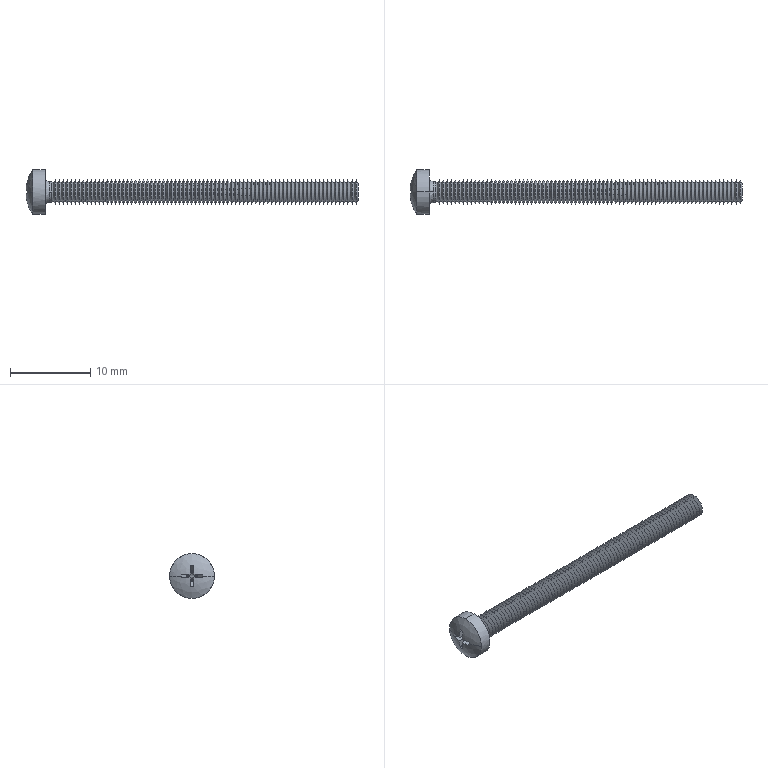Part | SolidWorks | features BaseBody 1 | 1 solid | 330 faces | box 41.388 x 5.6 x 5.6 mm | volume 251.599 mm3 | cone 308 | plane 14 | spline 4 | cylinder 4 | commonest cylinder face diameters 2.598 x2 5.6 x2